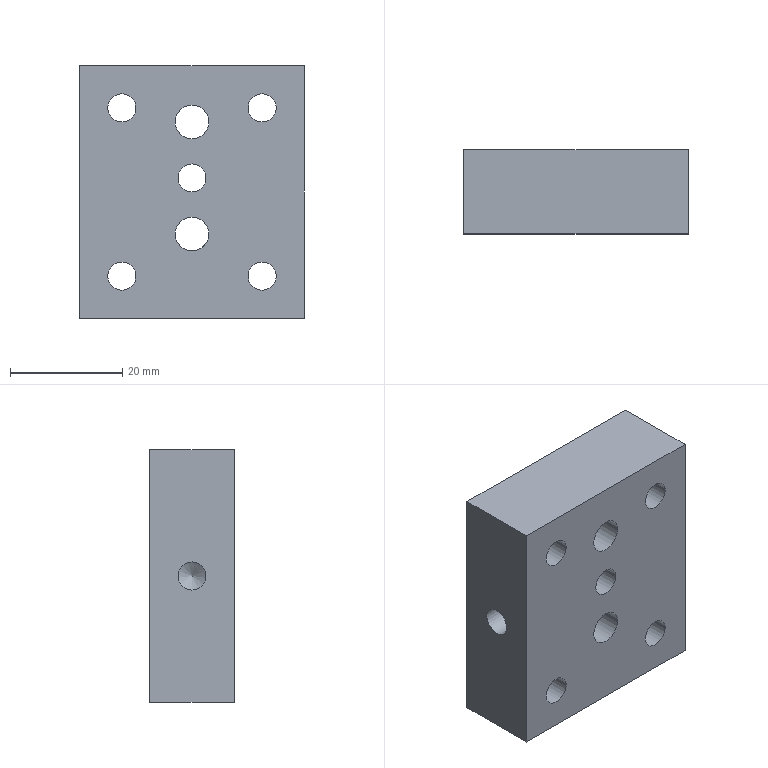Part | NX | features BREP 1 | 1 solid | 16 faces | box 40 x 15 x 45 mm | volume 24133 mm3 | cylinder 9 | plane 6 | cone 1 | commonest cylinder face diameters 5 x7 6 x2
STEP:
#1=CARTESIAN_POINT('',(20.,-7.5,22.5));
#2=VERTEX_POINT('',#1);
#3=CARTESIAN_POINT('',(20.,-7.5,-22.5));
#4=VERTEX_POINT('',#3);
#5=CARTESIAN_POINT('',(20.,-7.5,22.5));
#6=DIRECTION('',(0.,0.,-1.));
#7=VECTOR('',#6,1000.);
#8=LINE('',#5,#7);
#9=EDGE_CURVE('',#2,#4,#8,.T.);
#10=ORIENTED_EDGE('',*,*,#9,.T.);
#11=CARTESIAN_POINT('',(20.,7.5,-22.5));
#12=VERTEX_POINT('',#11);
#13=CARTESIAN_POINT('',(20.,7.5,-22.5));
#14=DIRECTION('',(0.,-1.,0.));
#15=VECTOR('',#14,1000.);
#16=LINE('',#13,#15);
#17=EDGE_CURVE('',#12,#4,#16,.T.);
#18=ORIENTED_EDGE('',*,*,#17,.F.);
#19=CARTESIAN_POINT('',(20.,7.5,22.5));
#20=VERTEX_POINT('',#19);
#21=CARTESIAN_POINT('',(20.,7.5,22.5));
#22=DIRECTION('',(0.,0.,-1.));
#23=VECTOR('',#22,1000.);
#24=LINE('',#21,#23);
#25=EDGE_CURVE('',#20,#12,#24,.T.);
#26=ORIENTED_EDGE('',*,*,#25,.F.);
#27=CARTESIAN_POINT('',(20.,7.5,22.5));
#28=DIRECTION('',(0.,-1.,0.));
#29=VECTOR('',#28,1000.);
#30=LINE('',#27,#29);
#31=EDGE_CURVE('',#20,#2,#30,.T.);
#32=ORIENTED_EDGE('',*,*,#31,.T.);
#33=EDGE_LOOP('',(#10,#18,#26,#32));
#34=FACE_BOUND('',#33,.T.);
#35=CARTESIAN_POINT('',(20.,7.5,22.5));
#36=DIRECTION('',(-1.,0.,0.));
#37=DIRECTION('',(0.,0.,-1.));
#38=AXIS2_PLACEMENT_3D('',#35,#36,#37);
#39=PLANE('',#38);
#40=ADVANCED_FACE('',(#34),#39,.F.);
#41=CARTESIAN_POINT('',(-2.5,0.,-22.5));
#42=VERTEX_POINT('',#41);
#43=CARTESIAN_POINT('',(0.,0.,-22.5));
#44=DIRECTION('',(0.,0.,-1.));
#45=DIRECTION('',(-1.,0.,0.));
#46=AXIS2_PLACEMENT_3D('',#43,#44,#45);
#47=CIRCLE('',#46,2.5);
#48=EDGE_CURVE('',#42,#42,#47,.T.);
#49=ORIENTED_EDGE('',*,*,#48,.F.);
#50=EDGE_LOOP('',(#49));
#51=FACE_BOUND('',#50,.T.);
#52=CARTESIAN_POINT('',(-20.,-7.5,-22.5));
#53=VERTEX_POINT('',#52);
#54=CARTESIAN_POINT('',(-20.,-7.5,-22.5));
#55=DIRECTION('',(-1.,0.,0.));
#56=VECTOR('',#55,1000.);
#57=LINE('',#54,#56);
#58=EDGE_CURVE('',#4,#53,#57,.T.);
#59=ORIENTED_EDGE('',*,*,#58,.T.);
#60=CARTESIAN_POINT('',(-20.,7.5,-22.5));
#61=VERTEX_POINT('',#60);
#62=CARTESIAN_POINT('',(-20.,7.5,-22.5));
#63=DIRECTION('',(0.,-1.,0.));
#64=VECTOR('',#63,1000.);
#65=LINE('',#62,#64);
#66=EDGE_CURVE('',#61,#53,#65,.T.);
#67=ORIENTED_EDGE('',*,*,#66,.F.);
#68=CARTESIAN_POINT('',(-20.,7.5,-22.5));
#69=DIRECTION('',(-1.,0.,0.));
#70=VECTOR('',#69,1000.);
#71=LINE('',#68,#70);
#72=EDGE_CURVE('',#12,#61,#71,.T.);
#73=ORIENTED_EDGE('',*,*,#72,.F.);
#74=ORIENTED_EDGE('',*,*,#17,.T.);
#75=EDGE_LOOP('',(#59,#67,#73,#74));
#76=FACE_BOUND('',#75,.T.);
#77=CARTESIAN_POINT('',(-20.,7.5,-22.5));
#78=DIRECTION('',(0.,0.,1.));
#79=DIRECTION('',(-1.,0.,0.));
#80=AXIS2_PLACEMENT_3D('',#77,#78,#79);
#81=PLANE('',#80);
#82=ADVANCED_FACE('',(#51,#76),#81,.F.);
#83=CARTESIAN_POINT('',(-20.,0.,2.5));
#84=VERTEX_POINT('',#83);
#85=CARTESIAN_POINT('',(-20.,0.,0.));
#86=DIRECTION('',(-1.,0.,0.));
#87=DIRECTION('',(0.,0.,1.));
#88=AXIS2_PLACEMENT_3D('',#85,#86,#87);
#89=CIRCLE('',#88,2.5);
#90=EDGE_CURVE('',#84,#84,#89,.T.);
#91=ORIENTED_EDGE('',*,*,#90,.F.);
#92=EDGE_LOOP('',(#91));
#93=FACE_BOUND('',#92,.T.);
#94=CARTESIAN_POINT('',(-20.,-7.5,22.5));
#95=VERTEX_POINT('',#94);
#96=CARTESIAN_POINT('',(-20.,-7.5,22.5));
#97=DIRECTION('',(0.,0.,1.));
#98=VECTOR('',#97,1000.);
#99=LINE('',#96,#98);
#100=EDGE_CURVE('',#53,#95,#99,.T.);
#101=ORIENTED_EDGE('',*,*,#100,.T.);
#102=CARTESIAN_POINT('',(-20.,7.5,22.5));
#103=VERTEX_POINT('',#102);
#104=CARTESIAN_POINT('',(-20.,7.5,22.5));
#105=DIRECTION('',(0.,-1.,0.));
#106=VECTOR('',#105,1000.);
#107=LINE('',#104,#106);
#108=EDGE_CURVE('',#103,#95,#107,.T.);
#109=ORIENTED_EDGE('',*,*,#108,.F.);
#110=CARTESIAN_POINT('',(-20.,7.5,22.5));
#111=DIRECTION('',(0.,0.,1.));
#112=VECTOR('',#111,1000.);
#113=LINE('',#110,#112);
#114=EDGE_CURVE('',#61,#103,#113,.T.);
#115=ORIENTED_EDGE('',*,*,#114,.F.);
#116=ORIENTED_EDGE('',*,*,#66,.T.);
#117=EDGE_LOOP('',(#101,#109,#115,#116));
#118=FACE_BOUND('',#117,.T.);
#119=CARTESIAN_POINT('',(-20.,7.5,22.5));
#120=DIRECTION('',(1.,0.,0.));
#121=DIRECTION('',(0.,0.,1.));
#122=AXIS2_PLACEMENT_3D('',#119,#120,#121);
#123=PLANE('',#122);
#124=ADVANCED_FACE('',(#93,#118),#123,.F.);
#125=CARTESIAN_POINT('',(-20.,-7.5,22.5));
#126=DIRECTION('',(1.,0.,0.));
#127=VECTOR('',#126,1000.);
#128=LINE('',#125,#127);
#129=EDGE_CURVE('',#95,#2,#128,.T.);
#130=ORIENTED_EDGE('',*,*,#129,.T.);
#131=ORIENTED_EDGE('',*,*,#31,.F.);
#132=CARTESIAN_POINT('',(-20.,7.5,22.5));
#133=DIRECTION('',(1.,0.,0.));
#134=VECTOR('',#133,1000.);
#135=LINE('',#132,#134);
#136=EDGE_CURVE('',#103,#20,#135,.T.);
#137=ORIENTED_EDGE('',*,*,#136,.F.);
#138=ORIENTED_EDGE('',*,*,#108,.T.);
#139=EDGE_LOOP('',(#130,#131,#137,#138));
#140=FACE_BOUND('',#139,.T.);
#141=CARTESIAN_POINT('',(-20.,7.5,22.5));
#142=DIRECTION('',(0.,0.,-1.));
#143=DIRECTION('',(1.,0.,0.));
#144=AXIS2_PLACEMENT_3D('',#141,#142,#143);
#145=PLANE('',#144);
#146=ADVANCED_FACE('',(#140),#145,.F.);
#147=CARTESIAN_POINT('',(12.5,7.5,-17.5));
#148=VERTEX_POINT('',#147);
#149=CARTESIAN_POINT('',(12.5,7.5,-15.));
#150=DIRECTION('',(0.,-1.,0.));
#151=DIRECTION('',(0.,0.,-1.));
#152=AXIS2_PLACEMENT_3D('',#149,#150,#151);
#153=CIRCLE('',#152,2.5);
#154=EDGE_CURVE('',#148,#148,#153,.T.);
#155=ORIENTED_EDGE('',*,*,#154,.T.);
#156=EDGE_LOOP('',(#155));
#157=FACE_BOUND('',#156,.T.);
#158=CARTESIAN_POINT('',(-12.5,7.5,12.5));
#159=VERTEX_POINT('',#158);
#160=CARTESIAN_POINT('',(-12.5,7.5,15.));
#161=DIRECTION('',(0.,-1.,0.));
#162=DIRECTION('',(0.,0.,-1.));
#163=AXIS2_PLACEMENT_3D('',#160,#161,#162);
#164=CIRCLE('',#163,2.5);
#165=EDGE_CURVE('',#159,#159,#164,.T.);
#166=ORIENTED_EDGE('',*,*,#165,.T.);
#167=EDGE_LOOP('',(#166));
#168=FACE_BOUND('',#167,.T.);
#169=CARTESIAN_POINT('',(12.5,7.5,12.5));
#170=VERTEX_POINT('',#169);
#171=CARTESIAN_POINT('',(12.5,7.5,15.));
#172=DIRECTION('',(0.,-1.,0.));
#173=DIRECTION('',(0.,0.,-1.));
#174=AXIS2_PLACEMENT_3D('',#171,#172,#173);
#175=CIRCLE('',#174,2.5);
#176=EDGE_CURVE('',#170,#170,#175,.T.);
#177=ORIENTED_EDGE('',*,*,#176,.T.);
#178=EDGE_LOOP('',(#177));
#179=FACE_BOUND('',#178,.T.);
#180=CARTESIAN_POINT('',(-12.5,7.5,-17.5));
#181=VERTEX_POINT('',#180);
#182=CARTESIAN_POINT('',(-12.5,7.5,-15.));
#183=DIRECTION('',(0.,-1.,0.));
#184=DIRECTION('',(0.,0.,-1.));
#185=AXIS2_PLACEMENT_3D('',#182,#183,#184);
#186=CIRCLE('',#185,2.5);
#187=EDGE_CURVE('',#181,#181,#186,.T.);
#188=ORIENTED_EDGE('',*,*,#187,.T.);
#189=EDGE_LOOP('',(#188));
#190=FACE_BOUND('',#189,.T.);
#191=CARTESIAN_POINT('',(0.,7.5,5.));
#192=VERTEX_POINT('',#191);
#193=CARTESIAN_POINT('',(0.,7.5,2.5));
#194=DIRECTION('',(0.,1.,0.));
#195=DIRECTION('',(0.,0.,1.));
#196=AXIS2_PLACEMENT_3D('',#193,#194,#195);
#197=CIRCLE('',#196,2.5);
#198=EDGE_CURVE('',#192,#192,#197,.T.);
#199=ORIENTED_EDGE('',*,*,#198,.F.);
#200=EDGE_LOOP('',(#199));
#201=FACE_BOUND('',#200,.T.);
#202=CARTESIAN_POINT('',(0.,7.5,-4.5));
#203=VERTEX_POINT('',#202);
#204=CARTESIAN_POINT('',(0.,7.5,-7.5));
#205=DIRECTION('',(0.,1.,0.));
#206=DIRECTION('',(0.,0.,1.));
#207=AXIS2_PLACEMENT_3D('',#204,#205,#206);
#208=CIRCLE('',#207,3.);
#209=EDGE_CURVE('',#203,#203,#208,.T.);
#210=ORIENTED_EDGE('',*,*,#209,.F.);
#211=EDGE_LOOP('',(#210));
#212=FACE_BOUND('',#211,.T.);
#213=CARTESIAN_POINT('',(0.,7.5,15.5));
#214=VERTEX_POINT('',#213);
#215=CARTESIAN_POINT('',(0.,7.5,12.5));
#216=DIRECTION('',(0.,1.,0.));
#217=DIRECTION('',(0.,0.,1.));
#218=AXIS2_PLACEMENT_3D('',#215,#216,#217);
#219=CIRCLE('',#218,3.);
#220=EDGE_CURVE('',#214,#214,#219,.T.);
#221=ORIENTED_EDGE('',*,*,#220,.F.);
#222=EDGE_LOOP('',(#221));
#223=FACE_BOUND('',#222,.T.);
#224=ORIENTED_EDGE('',*,*,#25,.T.);
#225=ORIENTED_EDGE('',*,*,#72,.T.);
#226=ORIENTED_EDGE('',*,*,#114,.T.);
#227=ORIENTED_EDGE('',*,*,#136,.T.);
#228=EDGE_LOOP('',(#224,#225,#226,#227));
#229=FACE_BOUND('',#228,.T.);
#230=CARTESIAN_POINT('',(0.,7.5,0.));
#231=DIRECTION('',(0.,-1.,0.));
#232=DIRECTION('',(0.,0.,1.));
#233=AXIS2_PLACEMENT_3D('',#230,#231,#232);
#234=PLANE('',#233);
#235=ADVANCED_FACE('',(#157,#168,#179,#190,#201,#212,#223,#229),#234,.F.);
#236=CARTESIAN_POINT('',(12.5,-7.5,-17.5));
#237=VERTEX_POINT('',#236);
#238=CARTESIAN_POINT('',(12.5,-7.5,-15.));
#239=DIRECTION('',(0.,-1.,0.));
#240=DIRECTION('',(0.,0.,-1.));
#241=AXIS2_PLACEMENT_3D('',#238,#239,#240);
#242=CIRCLE('',#241,2.5);
#243=EDGE_CURVE('',#237,#237,#242,.T.);
#244=ORIENTED_EDGE('',*,*,#243,.F.);
#245=EDGE_LOOP('',(#244));
#246=FACE_BOUND('',#245,.T.);
#247=CARTESIAN_POINT('',(-12.5,-7.5,12.5));
#248=VERTEX_POINT('',#247);
#249=CARTESIAN_POINT('',(-12.5,-7.5,15.));
#250=DIRECTION('',(0.,-1.,0.));
#251=DIRECTION('',(0.,0.,-1.));
#252=AXIS2_PLACEMENT_3D('',#249,#250,#251);
#253=CIRCLE('',#252,2.5);
#254=EDGE_CURVE('',#248,#248,#253,.T.);
#255=ORIENTED_EDGE('',*,*,#254,.F.);
#256=EDGE_LOOP('',(#255));
#257=FACE_BOUND('',#256,.T.);
#258=CARTESIAN_POINT('',(12.5,-7.5,12.5));
#259=VERTEX_POINT('',#258);
#260=CARTESIAN_POINT('',(12.5,-7.5,15.));
#261=DIRECTION('',(0.,-1.,0.));
#262=DIRECTION('',(0.,0.,-1.));
#263=AXIS2_PLACEMENT_3D('',#260,#261,#262);
#264=CIRCLE('',#263,2.5);
#265=EDGE_CURVE('',#259,#259,#264,.T.);
#266=ORIENTED_EDGE('',*,*,#265,.F.);
#267=EDGE_LOOP('',(#266));
#268=FACE_BOUND('',#267,.T.);
#269=CARTESIAN_POINT('',(-12.5,-7.5,-17.5));
#270=VERTEX_POINT('',#269);
#271=CARTESIAN_POINT('',(-12.5,-7.5,-15.));
#272=DIRECTION('',(0.,-1.,0.));
#273=DIRECTION('',(0.,0.,-1.));
#274=AXIS2_PLACEMENT_3D('',#271,#272,#273);
#275=CIRCLE('',#274,2.5);
#276=EDGE_CURVE('',#270,#270,#275,.T.);
#277=ORIENTED_EDGE('',*,*,#276,.F.);
#278=EDGE_LOOP('',(#277));
#279=FACE_BOUND('',#278,.T.);
#280=CARTESIAN_POINT('',(0.,-7.5,5.));
#281=VERTEX_POINT('',#280);
#282=CARTESIAN_POINT('',(0.,-7.5,2.5));
#283=DIRECTION('',(0.,1.,0.));
#284=DIRECTION('',(0.,0.,1.));
#285=AXIS2_PLACEMENT_3D('',#282,#283,#284);
#286=CIRCLE('',#285,2.5);
#287=EDGE_CURVE('',#281,#281,#286,.T.);
#288=ORIENTED_EDGE('',*,*,#287,.T.);
#289=EDGE_LOOP('',(#288));
#290=FACE_BOUND('',#289,.T.);
#291=CARTESIAN_POINT('',(0.,-7.5,-4.5));
#292=VERTEX_POINT('',#291);
#293=CARTESIAN_POINT('',(0.,-7.5,-7.5));
#294=DIRECTION('',(0.,1.,0.));
#295=DIRECTION('',(0.,0.,1.));
#296=AXIS2_PLACEMENT_3D('',#293,#294,#295);
#297=CIRCLE('',#296,3.);
#298=EDGE_CURVE('',#292,#292,#297,.T.);
#299=ORIENTED_EDGE('',*,*,#298,.T.);
#300=EDGE_LOOP('',(#299));
#301=FACE_BOUND('',#300,.T.);
#302=CARTESIAN_POINT('',(0.,-7.5,15.5));
#303=VERTEX_POINT('',#302);
#304=CARTESIAN_POINT('',(0.,-7.5,12.5));
#305=DIRECTION('',(0.,1.,0.));
#306=DIRECTION('',(0.,0.,1.));
#307=AXIS2_PLACEMENT_3D('',#304,#305,#306);
#308=CIRCLE('',#307,3.);
#309=EDGE_CURVE('',#303,#303,#308,.T.);
#310=ORIENTED_EDGE('',*,*,#309,.T.);
#311=EDGE_LOOP('',(#310));
#312=FACE_BOUND('',#311,.T.);
#313=ORIENTED_EDGE('',*,*,#9,.F.);
#314=ORIENTED_EDGE('',*,*,#129,.F.);
#315=ORIENTED_EDGE('',*,*,#100,.F.);
#316=ORIENTED_EDGE('',*,*,#58,.F.);
#317=EDGE_LOOP('',(#313,#314,#315,#316));
#318=FACE_BOUND('',#317,.T.);
#319=CARTESIAN_POINT('',(0.,-7.5,0.));
#320=DIRECTION('',(0.,-1.,0.));
#321=DIRECTION('',(0.,0.,1.));
#322=AXIS2_PLACEMENT_3D('',#319,#320,#321);
#323=PLANE('',#322);
#324=ADVANCED_FACE('',(#246,#257,#268,#279,#290,#301,#312,#318),#323,.T.);
#325=CARTESIAN_POINT('',(-3.498,0.,0.));
#326=VERTEX_POINT('',#325);
#327=VERTEX_LOOP('',#326);
#328=FACE_BOUND('',#327,.T.);
#329=CARTESIAN_POINT('',(-5.,0.,2.5));
#330=VERTEX_POINT('',#329);
#331=CARTESIAN_POINT('',(-5.,0.,0.));
#332=DIRECTION('',(-1.,0.,0.));
#333=DIRECTION('',(0.,0.,1.));
#334=AXIS2_PLACEMENT_3D('',#331,#332,#333);
#335=CIRCLE('',#334,2.5);
#336=EDGE_CURVE('',#330,#330,#335,.T.);
#337=ORIENTED_EDGE('',*,*,#336,.T.);
#338=EDGE_LOOP('',(#337));
#339=FACE_BOUND('',#338,.T.);
#340=CARTESIAN_POINT('',(-5.,0.,0.));
#341=DIRECTION('',(-1.,0.,0.));
#342=DIRECTION('',(0.,0.,-1.));
#343=AXIS2_PLACEMENT_3D('',#340,#341,#342);
#344=CONICAL_SURFACE('',#343,2.5,1.03);
#345=ADVANCED_FACE('',(#328,#339),#344,.F.);
#346=ORIENTED_EDGE('',*,*,#336,.F.);
#347=EDGE_LOOP('',(#346));
#348=FACE_BOUND('',#347,.T.);
#349=ORIENTED_EDGE('',*,*,#90,.T.);
#350=EDGE_LOOP('',(#349));
#351=FACE_BOUND('',#350,.T.);
#352=CARTESIAN_POINT('',(-20.,0.,0.));
#353=DIRECTION('',(-1.,0.,0.));
#354=DIRECTION('',(0.,0.,-1.));
#355=AXIS2_PLACEMENT_3D('',#352,#353,#354);
#356=CYLINDRICAL_SURFACE('',#355,2.5);
#357=ADVANCED_FACE('',(#348,#351),#356,.F.);
#358=CARTESIAN_POINT('',(-2.5,0.,-9.158));
#359=VERTEX_POINT('',#358);
#360=CARTESIAN_POINT('',(-2.347,1.029,-9.401));
#361=CARTESIAN_POINT('',(-2.576,-0.001174,-9.037));
#362=CARTESIAN_POINT('',(-2.348,-1.024,-9.399));
#363=CARTESIAN_POINT('',(-1.834,-1.777,-9.92));
#364=CARTESIAN_POINT('',(-1.048,-2.345,-10.369));
#365=CARTESIAN_POINT('',(-0.003619,-2.577,-10.565));
#366=CARTESIAN_POINT('',(1.041,-2.348,-10.371));
#367=CARTESIAN_POINT('',(1.832,-1.78,-9.923));
#368=CARTESIAN_POINT('',(2.347,-1.027,-9.401));
#369=CARTESIAN_POINT('',(2.576,-0.0005699,-9.038));
#370=CARTESIAN_POINT('',(2.349,1.023,-9.398));
#371=CARTESIAN_POINT('',(1.833,1.778,-9.921));
#372=CARTESIAN_POINT('',(1.053,2.342,-10.366));
#373=CARTESIAN_POINT('',(0.008018,2.577,-10.565));
#374=CARTESIAN_POINT('',(-1.04,2.349,-10.372));
#375=CARTESIAN_POINT('',(-1.831,1.781,-9.924));
#376=CARTESIAN_POINT('',(-2.347,1.029,-9.401));
#377=CARTESIAN_POINT('',(-2.576,-0.001174,-9.037));
#378=CARTESIAN_POINT('',(-2.348,-1.024,-9.399));
#379=B_SPLINE_CURVE_WITH_KNOTS('',3,(#360,#361,#362,#363,#364,#365,#366,#367,#368,#369,#370,#371,#372,#373,#374,#375,#376,#377,#378),.UNSPECIFIED.,.T.,.F.,(1,1,1,1,1,1,1,1,1,1,1,1,1,1,1,1,1,1,1,1,1,1,1),(-0.003136,-0.002091,-0.001045,0.,0.001045,0.002091,0.003136,0.004181,0.005226,0.006272,0.007317,0.008362,0.009408,0.01045,0.0115,0.01254,0.01359,0.01463,0.01568,0.01672,0.01777,0.01882,0.01986),.UNSPECIFIED.);
#380=EDGE_CURVE('',#359,#359,#379,.T.);
#381=ORIENTED_EDGE('',*,*,#380,.T.);
#382=EDGE_LOOP('',(#381));
#383=FACE_BOUND('',#382,.T.);
#384=ORIENTED_EDGE('',*,*,#48,.T.);
#385=EDGE_LOOP('',(#384));
#386=FACE_BOUND('',#385,.T.);
#387=CARTESIAN_POINT('',(0.,0.,-22.5));
#388=DIRECTION('',(0.,0.,-1.));
#389=DIRECTION('',(1.,0.,0.));
#390=AXIS2_PLACEMENT_3D('',#387,#388,#389);
#391=CYLINDRICAL_SURFACE('',#390,2.5);
#392=ADVANCED_FACE('',(#383,#386),#391,.F.);
#393=ORIENTED_EDGE('',*,*,#309,.F.);
#394=EDGE_LOOP('',(#393));
#395=FACE_BOUND('',#394,.T.);
#396=ORIENTED_EDGE('',*,*,#220,.T.);
#397=EDGE_LOOP('',(#396));
#398=FACE_BOUND('',#397,.T.);
#399=CARTESIAN_POINT('',(0.,7.5,12.5));
#400=DIRECTION('',(0.,1.,0.));
#401=DIRECTION('',(0.,0.,-1.));
#402=AXIS2_PLACEMENT_3D('',#399,#400,#401);
#403=CYLINDRICAL_SURFACE('',#402,3.);
#404=ADVANCED_FACE('',(#395,#398),#403,.F.);
#405=ORIENTED_EDGE('',*,*,#209,.T.);
#406=EDGE_LOOP('',(#405));
#407=FACE_BOUND('',#406,.T.);
#408=ORIENTED_EDGE('',*,*,#298,.F.);
#409=EDGE_LOOP('',(#408));
#410=FACE_BOUND('',#409,.T.);
#411=ORIENTED_EDGE('',*,*,#380,.F.);
#412=EDGE_LOOP('',(#411));
#413=FACE_BOUND('',#412,.T.);
#414=CARTESIAN_POINT('',(0.,7.5,-7.5));
#415=DIRECTION('',(0.,1.,0.));
#416=DIRECTION('',(0.,0.,-1.));
#417=AXIS2_PLACEMENT_3D('',#414,#415,#416);
#418=CYLINDRICAL_SURFACE('',#417,3.);
#419=ADVANCED_FACE('',(#407,#410,#413),#418,.F.);
#420=ORIENTED_EDGE('',*,*,#287,.F.);
#421=EDGE_LOOP('',(#420));
#422=FACE_BOUND('',#421,.T.);
#423=ORIENTED_EDGE('',*,*,#198,.T.);
#424=EDGE_LOOP('',(#423));
#425=FACE_BOUND('',#424,.T.);
#426=CARTESIAN_POINT('',(0.,7.5,2.5));
#427=DIRECTION('',(0.,1.,0.));
#428=DIRECTION('',(0.,0.,-1.));
#429=AXIS2_PLACEMENT_3D('',#426,#427,#428);
#430=CYLINDRICAL_SURFACE('',#429,2.5);
#431=ADVANCED_FACE('',(#422,#425),#430,.F.);
#432=ORIENTED_EDGE('',*,*,#187,.F.);
#433=EDGE_LOOP('',(#432));
#434=FACE_BOUND('',#433,.T.);
#435=ORIENTED_EDGE('',*,*,#276,.T.);
#436=EDGE_LOOP('',(#435));
#437=FACE_BOUND('',#436,.T.);
#438=CARTESIAN_POINT('',(-12.5,-7.5,-15.));
#439=DIRECTION('',(0.,-1.,0.));
#440=DIRECTION('',(0.,0.,1.));
#441=AXIS2_PLACEMENT_3D('',#438,#439,#440);
#442=CYLINDRICAL_SURFACE('',#441,2.5);
#443=ADVANCED_FACE('',(#434,#437),#442,.F.);
#444=ORIENTED_EDGE('',*,*,#176,.F.);
#445=EDGE_LOOP('',(#444));
#446=FACE_BOUND('',#445,.T.);
#447=ORIENTED_EDGE('',*,*,#265,.T.);
#448=EDGE_LOOP('',(#447));
#449=FACE_BOUND('',#448,.T.);
#450=CARTESIAN_POINT('',(12.5,-7.5,15.));
#451=DIRECTION('',(0.,-1.,0.));
#452=DIRECTION('',(0.,0.,1.));
#453=AXIS2_PLACEMENT_3D('',#450,#451,#452);
#454=CYLINDRICAL_SURFACE('',#453,2.5);
#455=ADVANCED_FACE('',(#446,#449),#454,.F.);
#456=ORIENTED_EDGE('',*,*,#165,.F.);
#457=EDGE_LOOP('',(#456));
#458=FACE_BOUND('',#457,.T.);
#459=ORIENTED_EDGE('',*,*,#254,.T.);
#460=EDGE_LOOP('',(#459));
#461=FACE_BOUND('',#460,.T.);
#462=CARTESIAN_POINT('',(-12.5,-7.5,15.));
#463=DIRECTION('',(0.,-1.,0.));
#464=DIRECTION('',(0.,0.,1.));
#465=AXIS2_PLACEMENT_3D('',#462,#463,#464);
#466=CYLINDRICAL_SURFACE('',#465,2.5);
#467=ADVANCED_FACE('',(#458,#461),#466,.F.);
#468=ORIENTED_EDGE('',*,*,#154,.F.);
#469=EDGE_LOOP('',(#468));
#470=FACE_BOUND('',#469,.T.);
#471=ORIENTED_EDGE('',*,*,#243,.T.);
#472=EDGE_LOOP('',(#471));
#473=FACE_BOUND('',#472,.T.);
#474=CARTESIAN_POINT('',(12.5,-7.5,-15.));
#475=DIRECTION('',(0.,-1.,0.));
#476=DIRECTION('',(0.,0.,1.));
#477=AXIS2_PLACEMENT_3D('',#474,#475,#476);
#478=CYLINDRICAL_SURFACE('',#477,2.5);
#479=ADVANCED_FACE('',(#470,#473),#478,.F.);
#480=CLOSED_SHELL('',(#40,#82,#124,#146,#235,#324,#345,#357,#392,#404,#419,#431,#443,#455,#467,#479));
#481=MANIFOLD_SOLID_BREP('',#480);
#482=(LENGTH_UNIT()NAMED_UNIT(*)SI_UNIT(.MILLI.,.METRE.));
#483=UNCERTAINTY_MEASURE_WITH_UNIT(LENGTH_MEASURE(0.0508),#482,'','');
#484=(NAMED_UNIT(*)PLANE_ANGLE_UNIT()SI_UNIT($,.RADIAN.));
#485=(NAMED_UNIT(*)SI_UNIT($,.STERADIAN.)SOLID_ANGLE_UNIT());
#486=(GEOMETRIC_REPRESENTATION_CONTEXT(3)GLOBAL_UNCERTAINTY_ASSIGNED_CONTEXT((#483))GLOBAL_UNIT_ASSIGNED_CONTEXT((#482,#484,#485))REPRESENTATION_CONTEXT('',''));
#487=ADVANCED_BREP_SHAPE_REPRESENTATION('',(#481),#486);